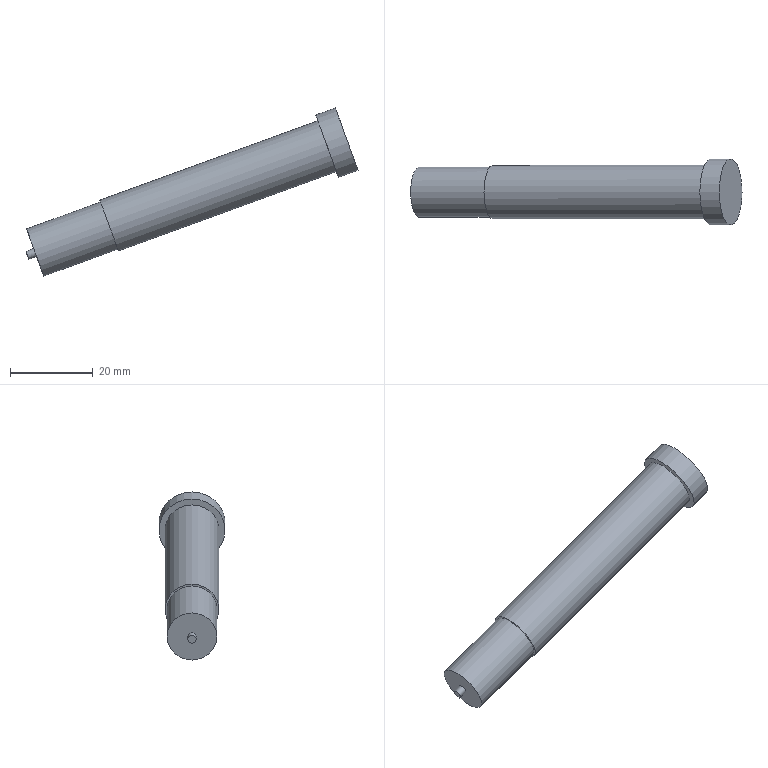Part | NX | features solid 2 | 1 solid | 9 faces | box 80.133 x 16 x 40.564 mm | volume 10629 mm3 | plane 5 | cylinder 4 | commonest cylinder face diameters 2 x1 12.1 x1 13 x1 16 x1
STEP:
#1=CARTESIAN_POINT('',(-603.95,-131.418,-2.151));
#2=VERTEX_POINT('',#1);
#3=CARTESIAN_POINT('',(-601.727,-131.418,-8.259));
#4=DIRECTION('',(-0.9397,0.,-0.342));
#5=DIRECTION('',(-0.342,0.,0.9397));
#6=AXIS2_PLACEMENT_3D('',#3,#4,#5);
#7=CIRCLE('',#6,6.5);
#8=EDGE_CURVE('',#2,#2,#7,.T.);
#9=ORIENTED_EDGE('',*,*,#8,.F.);
#10=EDGE_LOOP('',(#9));
#11=FACE_BOUND('',#10,.T.);
#12=CARTESIAN_POINT('',(-551.327,-131.418,17.002));
#13=VERTEX_POINT('',#12);
#14=CARTESIAN_POINT('',(-549.104,-131.418,10.894));
#15=DIRECTION('',(-0.9397,0.,-0.342));
#16=DIRECTION('',(-0.342,0.,0.9397));
#17=AXIS2_PLACEMENT_3D('',#14,#15,#16);
#18=CIRCLE('',#17,6.5);
#19=EDGE_CURVE('',#13,#13,#18,.T.);
#20=ORIENTED_EDGE('',*,*,#19,.T.);
#21=EDGE_LOOP('',(#20));
#22=FACE_BOUND('',#21,.T.);
#23=CARTESIAN_POINT('',(-544.406,-131.418,12.604));
#24=DIRECTION('',(-0.9397,0.,-0.342));
#25=DIRECTION('',(0.342,0.,-0.9397));
#26=AXIS2_PLACEMENT_3D('',#23,#24,#25);
#27=CYLINDRICAL_SURFACE('',#26,6.5);
#28=ADVANCED_FACE('',(#11,#22),#27,.T.);
#29=CARTESIAN_POINT('',(-603.796,-131.418,-2.574));
#30=VERTEX_POINT('',#29);
#31=CARTESIAN_POINT('',(-601.727,-131.418,-8.259));
#32=DIRECTION('',(-0.9397,0.,-0.342));
#33=DIRECTION('',(-0.342,0.,0.9397));
#34=AXIS2_PLACEMENT_3D('',#31,#32,#33);
#35=CIRCLE('',#34,6.05);
#36=EDGE_CURVE('',#30,#30,#35,.T.);
#37=ORIENTED_EDGE('',*,*,#36,.F.);
#38=EDGE_LOOP('',(#37));
#39=FACE_BOUND('',#38,.T.);
#40=ORIENTED_EDGE('',*,*,#8,.T.);
#41=EDGE_LOOP('',(#40));
#42=FACE_BOUND('',#41,.T.);
#43=CARTESIAN_POINT('',(-601.727,-131.418,-8.259));
#44=DIRECTION('',(0.9397,0.,0.342));
#45=DIRECTION('',(-0.342,0.,0.9397));
#46=AXIS2_PLACEMENT_3D('',#43,#44,#45);
#47=PLANE('',#46);
#48=ADVANCED_FACE('',(#39,#42),#47,.F.);
#49=CARTESIAN_POINT('',(-551.84,-131.418,18.411));
#50=VERTEX_POINT('',#49);
#51=CARTESIAN_POINT('',(-549.104,-131.418,10.894));
#52=DIRECTION('',(-0.9397,0.,-0.342));
#53=DIRECTION('',(-0.342,0.,0.9397));
#54=AXIS2_PLACEMENT_3D('',#51,#52,#53);
#55=CIRCLE('',#54,8.);
#56=EDGE_CURVE('',#50,#50,#55,.T.);
#57=ORIENTED_EDGE('',*,*,#56,.T.);
#58=EDGE_LOOP('',(#57));
#59=FACE_BOUND('',#58,.T.);
#60=ORIENTED_EDGE('',*,*,#19,.F.);
#61=EDGE_LOOP('',(#60));
#62=FACE_BOUND('',#61,.T.);
#63=CARTESIAN_POINT('',(-549.104,-131.418,10.894));
#64=DIRECTION('',(0.9397,0.,0.342));
#65=DIRECTION('',(-0.342,0.,0.9397));
#66=AXIS2_PLACEMENT_3D('',#63,#64,#65);
#67=PLANE('',#66);
#68=ADVANCED_FACE('',(#59,#62),#67,.F.);
#69=ORIENTED_EDGE('',*,*,#56,.F.);
#70=EDGE_LOOP('',(#69));
#71=FACE_BOUND('',#70,.T.);
#72=CARTESIAN_POINT('',(-547.142,-131.418,20.122));
#73=VERTEX_POINT('',#72);
#74=CARTESIAN_POINT('',(-544.406,-131.418,12.604));
#75=DIRECTION('',(-0.9397,0.,-0.342));
#76=DIRECTION('',(-0.342,0.,0.9397));
#77=AXIS2_PLACEMENT_3D('',#74,#75,#76);
#78=CIRCLE('',#77,8.);
#79=EDGE_CURVE('',#73,#73,#78,.T.);
#80=ORIENTED_EDGE('',*,*,#79,.T.);
#81=EDGE_LOOP('',(#80));
#82=FACE_BOUND('',#81,.T.);
#83=CARTESIAN_POINT('',(-549.104,-131.418,10.894));
#84=DIRECTION('',(0.9397,0.,0.342));
#85=DIRECTION('',(-0.342,0.,0.9397));
#86=AXIS2_PLACEMENT_3D('',#83,#84,#85);
#87=CYLINDRICAL_SURFACE('',#86,8.);
#88=ADVANCED_FACE('',(#71,#82),#87,.T.);
#89=ORIENTED_EDGE('',*,*,#79,.F.);
#90=EDGE_LOOP('',(#89));
#91=FACE_BOUND('',#90,.T.);
#92=CARTESIAN_POINT('',(-544.406,-131.418,12.604));
#93=DIRECTION('',(0.9397,0.,0.342));
#94=DIRECTION('',(-0.342,0.,0.9397));
#95=AXIS2_PLACEMENT_3D('',#92,#93,#94);
#96=PLANE('',#95);
#97=ADVANCED_FACE('',(#91),#96,.T.);
#98=CARTESIAN_POINT('',(-621.65,-131.418,-9.072));
#99=VERTEX_POINT('',#98);
#100=CARTESIAN_POINT('',(-619.581,-131.418,-14.758));
#101=DIRECTION('',(-0.9397,0.,-0.342));
#102=DIRECTION('',(-0.342,0.,0.9397));
#103=AXIS2_PLACEMENT_3D('',#100,#101,#102);
#104=CIRCLE('',#103,6.05);
#105=EDGE_CURVE('',#99,#99,#104,.T.);
#106=ORIENTED_EDGE('',*,*,#105,.F.);
#107=EDGE_LOOP('',(#106));
#108=FACE_BOUND('',#107,.T.);
#109=ORIENTED_EDGE('',*,*,#36,.T.);
#110=EDGE_LOOP('',(#109));
#111=FACE_BOUND('',#110,.T.);
#112=CARTESIAN_POINT('',(-619.581,-131.418,-14.758));
#113=DIRECTION('',(0.9397,0.,0.342));
#114=DIRECTION('',(-0.342,0.,0.9397));
#115=AXIS2_PLACEMENT_3D('',#112,#113,#114);
#116=CYLINDRICAL_SURFACE('',#115,6.05);
#117=ADVANCED_FACE('',(#108,#111),#116,.T.);
#118=CARTESIAN_POINT('',(-619.923,-131.418,-13.818));
#119=VERTEX_POINT('',#118);
#120=CARTESIAN_POINT('',(-619.581,-131.418,-14.758));
#121=DIRECTION('',(-0.9397,0.,-0.342));
#122=DIRECTION('',(-0.342,0.,0.9397));
#123=AXIS2_PLACEMENT_3D('',#120,#121,#122);
#124=CIRCLE('',#123,1.);
#125=EDGE_CURVE('',#119,#119,#124,.T.);
#126=ORIENTED_EDGE('',*,*,#125,.F.);
#127=EDGE_LOOP('',(#126));
#128=FACE_BOUND('',#127,.T.);
#129=ORIENTED_EDGE('',*,*,#105,.T.);
#130=EDGE_LOOP('',(#129));
#131=FACE_BOUND('',#130,.T.);
#132=CARTESIAN_POINT('',(-619.581,-131.418,-14.758));
#133=DIRECTION('',(0.9397,0.,0.342));
#134=DIRECTION('',(-0.342,0.,0.9397));
#135=AXIS2_PLACEMENT_3D('',#132,#133,#134);
#136=PLANE('',#135);
#137=ADVANCED_FACE('',(#128,#131),#136,.F.);
#138=CARTESIAN_POINT('',(-621.802,-131.418,-14.502));
#139=VERTEX_POINT('',#138);
#140=CARTESIAN_POINT('',(-621.46,-131.418,-15.442));
#141=DIRECTION('',(-0.9397,0.,-0.342));
#142=DIRECTION('',(-0.342,0.,0.9397));
#143=AXIS2_PLACEMENT_3D('',#140,#141,#142);
#144=CIRCLE('',#143,1.);
#145=EDGE_CURVE('',#139,#139,#144,.T.);
#146=ORIENTED_EDGE('',*,*,#145,.F.);
#147=EDGE_LOOP('',(#146));
#148=FACE_BOUND('',#147,.T.);
#149=ORIENTED_EDGE('',*,*,#125,.T.);
#150=EDGE_LOOP('',(#149));
#151=FACE_BOUND('',#150,.T.);
#152=CARTESIAN_POINT('',(-621.46,-131.418,-15.442));
#153=DIRECTION('',(0.9397,0.,0.342));
#154=DIRECTION('',(-0.342,0.,0.9397));
#155=AXIS2_PLACEMENT_3D('',#152,#153,#154);
#156=CYLINDRICAL_SURFACE('',#155,1.);
#157=ADVANCED_FACE('',(#148,#151),#156,.T.);
#158=ORIENTED_EDGE('',*,*,#145,.T.);
#159=EDGE_LOOP('',(#158));
#160=FACE_BOUND('',#159,.T.);
#161=CARTESIAN_POINT('',(-621.46,-131.418,-15.442));
#162=DIRECTION('',(0.9397,0.,0.342));
#163=DIRECTION('',(-0.342,0.,0.9397));
#164=AXIS2_PLACEMENT_3D('',#161,#162,#163);
#165=PLANE('',#164);
#166=ADVANCED_FACE('',(#160),#165,.F.);
#167=CLOSED_SHELL('',(#28,#48,#68,#88,#97,#117,#137,#157,#166));
#168=MANIFOLD_SOLID_BREP('',#167);
#169=(LENGTH_UNIT()NAMED_UNIT(*)SI_UNIT(.MILLI.,.METRE.));
#170=UNCERTAINTY_MEASURE_WITH_UNIT(LENGTH_MEASURE(0.00001),#169,'','');
#171=(NAMED_UNIT(*)PLANE_ANGLE_UNIT()SI_UNIT($,.RADIAN.));
#172=(NAMED_UNIT(*)SI_UNIT($,.STERADIAN.)SOLID_ANGLE_UNIT());
#173=(GEOMETRIC_REPRESENTATION_CONTEXT(3)GLOBAL_UNCERTAINTY_ASSIGNED_CONTEXT((#170))GLOBAL_UNIT_ASSIGNED_CONTEXT((#169,#171,#172))REPRESENTATION_CONTEXT('',''));
#174=ADVANCED_BREP_SHAPE_REPRESENTATION('',(#168),#173);